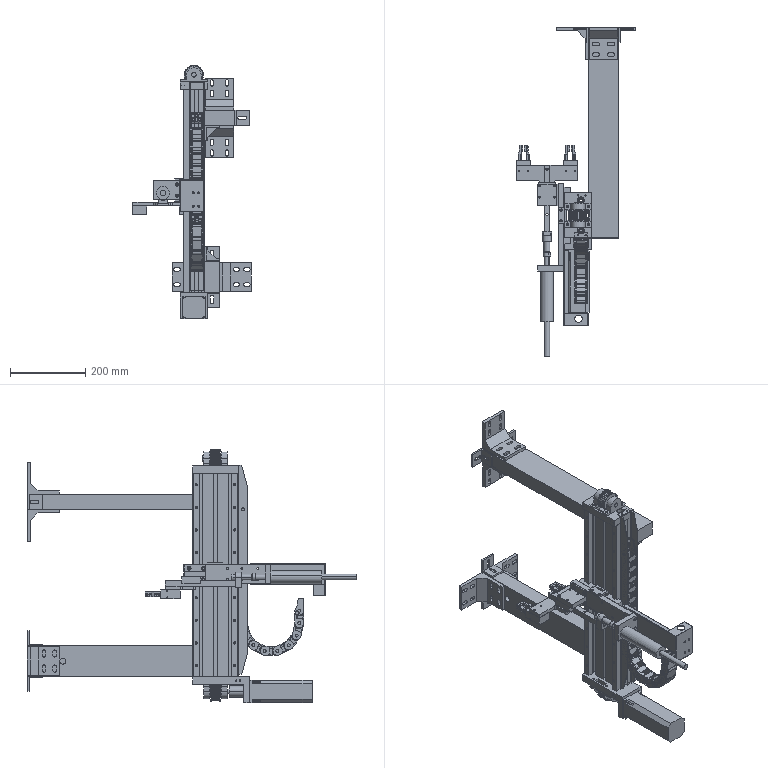Part | 78 solids | 4497 faces | volume 7661809 mm3 | plane 2322 | cylinder 2065 | cone 102 | torus 8 | commonest cylinder face diameters 2 x204 1 x170 0.96 x140 0.6 x136 3.3 x124 23.26 x119